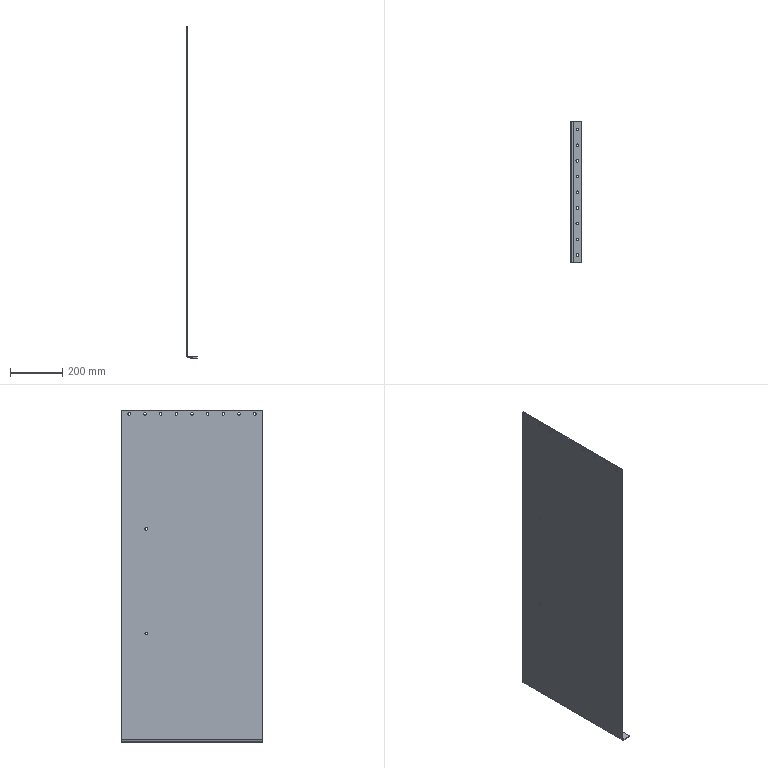Part | SolidWorks | features HoleWzd 3, LPattern 2, EdgeFlange 1, FlatPattern 1, MirrorPattern 1, SMBaseFlange 1, SheetMetal 1, UnFold 1, WeldmentFeature 1 | 1 solid | 54 faces | box 40 x 540 x 1270 mm | volume 2808187 mm3 | cylinder 42 | plane 12 | commonest cylinder face diameters 10 x41 18 x1